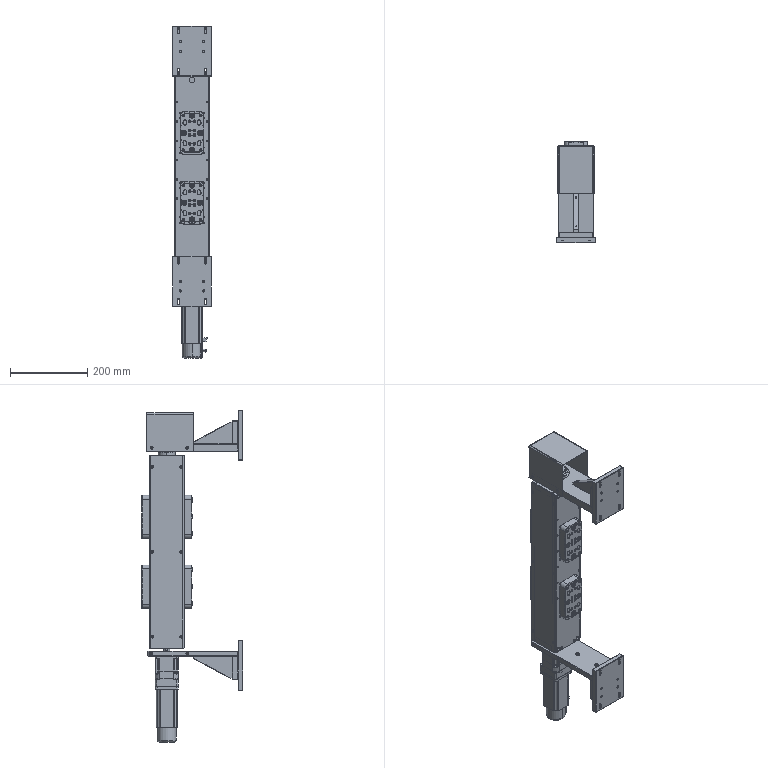Part | SolidWorks | features ReferencePattern 103, InContextFeatHolder 53, LocalLPattern 10, CompositeCurve 8, MirrorCompFeat 3, 3DProfileFeature 1, Attribute 1, LocalCirPattern 1 | 151 solids | 9498 faces | volume 4546068 mm3 | cylinder 3258 | plane 2980 | cone 2679 | spline 560 | torus 19 | sphere 2 | commonest cylinder face diameters 6 x401 2.5 x344 5 x197 9 x192 12 x187 11 x160